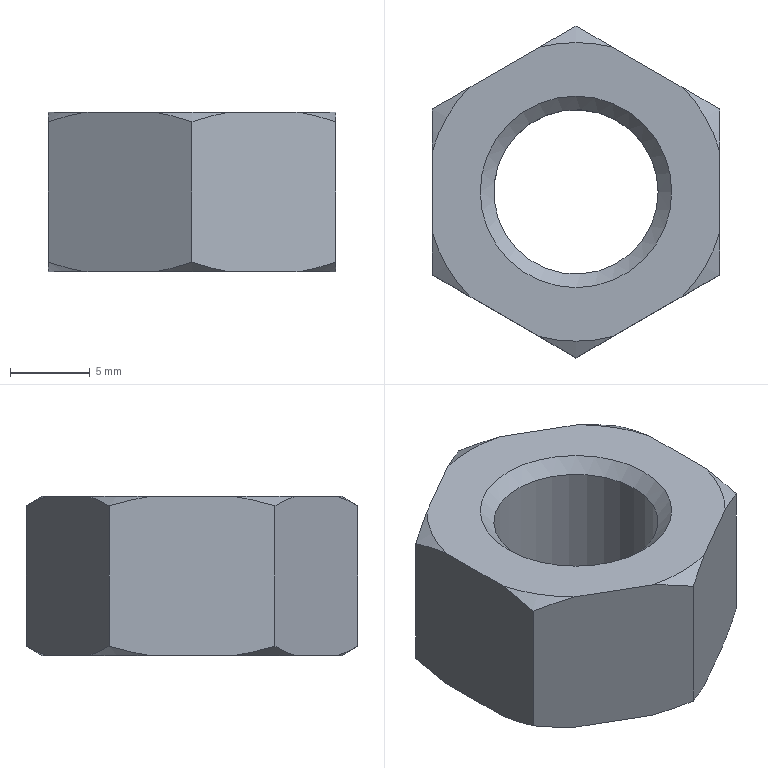Part | NX | features DATUM_CSYS 3, EXTRACT_FACE 2, EXTRACT_STRING 2, SKETCH 2, SWP104 2, EXTRUDE 1, HOLE PACKAGE 1, Instance Feature 1, Mirror Feature 1, SIMPLE HOLE 1, SYMBOLIC_THREAD 1 | 1 solid | 23 faces | box 18 x 20.785 x 10 mm | volume 1943 mm3 | cone 14 | plane 8 | cylinder 1 | commonest cylinder face diameters 10.3 x1
STEP:
#1=CARTESIAN_POINT('',(6.,0.,-10.));
#2=VERTEX_POINT('',#1);
#3=CARTESIAN_POINT('',(0.,0.,-10.));
#4=DIRECTION('',(0.,0.,1.));
#5=DIRECTION('',(1.,0.,0.));
#6=AXIS2_PLACEMENT_3D('',#3,#4,#5);
#7=CIRCLE('',#6,6.);
#8=EDGE_CURVE('',#2,#2,#7,.T.);
#9=ORIENTED_EDGE('',*,*,#8,.T.);
#10=EDGE_LOOP('',(#9));
#11=FACE_BOUND('',#10,.T.);
#12=CARTESIAN_POINT('',(9.,2.546,-10.));
#13=VERTEX_POINT('',#12);
#14=CARTESIAN_POINT('',(6.705,6.521,-10.));
#15=VERTEX_POINT('',#14);
#16=CARTESIAN_POINT('',(0.,0.,-10.));
#17=DIRECTION('',(0.,0.,1.));
#18=DIRECTION('',(1.,0.,0.));
#19=AXIS2_PLACEMENT_3D('',#16,#17,#18);
#20=CIRCLE('',#19,9.353);
#21=EDGE_CURVE('',#13,#15,#20,.T.);
#22=ORIENTED_EDGE('',*,*,#21,.F.);
#23=CARTESIAN_POINT('',(9.,-2.546,-10.));
#24=VERTEX_POINT('',#23);
#25=CARTESIAN_POINT('',(9.,-5.196,-10.));
#26=DIRECTION('',(0.,1.,0.));
#27=VECTOR('',#26,1000.);
#28=LINE('',#25,#27);
#29=EDGE_CURVE('',#24,#13,#28,.T.);
#30=ORIENTED_EDGE('',*,*,#29,.F.);
#31=CARTESIAN_POINT('',(6.705,-6.521,-10.));
#32=VERTEX_POINT('',#31);
#33=CARTESIAN_POINT('',(0.,0.,-10.));
#34=DIRECTION('',(0.,0.,1.));
#35=DIRECTION('',(1.,0.,0.));
#36=AXIS2_PLACEMENT_3D('',#33,#34,#35);
#37=CIRCLE('',#36,9.353);
#38=EDGE_CURVE('',#32,#24,#37,.T.);
#39=ORIENTED_EDGE('',*,*,#38,.F.);
#40=CARTESIAN_POINT('',(2.295,-9.067,-10.));
#41=VERTEX_POINT('',#40);
#42=CARTESIAN_POINT('',(0.,-10.392,-10.));
#43=DIRECTION('',(0.866,0.5,0.));
#44=VECTOR('',#43,1000.);
#45=LINE('',#42,#44);
#46=EDGE_CURVE('',#41,#32,#45,.T.);
#47=ORIENTED_EDGE('',*,*,#46,.F.);
#48=CARTESIAN_POINT('',(-2.295,-9.067,-10.));
#49=VERTEX_POINT('',#48);
#50=CARTESIAN_POINT('',(0.,0.,-10.));
#51=DIRECTION('',(0.,0.,1.));
#52=DIRECTION('',(1.,0.,0.));
#53=AXIS2_PLACEMENT_3D('',#50,#51,#52);
#54=CIRCLE('',#53,9.353);
#55=EDGE_CURVE('',#49,#41,#54,.T.);
#56=ORIENTED_EDGE('',*,*,#55,.F.);
#57=CARTESIAN_POINT('',(-6.705,-6.521,-10.));
#58=VERTEX_POINT('',#57);
#59=CARTESIAN_POINT('',(-9.,-5.196,-10.));
#60=DIRECTION('',(0.866,-0.5,0.));
#61=VECTOR('',#60,1000.);
#62=LINE('',#59,#61);
#63=EDGE_CURVE('',#58,#49,#62,.T.);
#64=ORIENTED_EDGE('',*,*,#63,.F.);
#65=CARTESIAN_POINT('',(-9.,-2.546,-10.));
#66=VERTEX_POINT('',#65);
#67=CARTESIAN_POINT('',(0.,0.,-10.));
#68=DIRECTION('',(0.,0.,1.));
#69=DIRECTION('',(1.,0.,0.));
#70=AXIS2_PLACEMENT_3D('',#67,#68,#69);
#71=CIRCLE('',#70,9.353);
#72=EDGE_CURVE('',#66,#58,#71,.T.);
#73=ORIENTED_EDGE('',*,*,#72,.F.);
#74=CARTESIAN_POINT('',(-9.,2.546,-10.));
#75=VERTEX_POINT('',#74);
#76=CARTESIAN_POINT('',(-9.,5.196,-10.));
#77=DIRECTION('',(0.,-1.,0.));
#78=VECTOR('',#77,1000.);
#79=LINE('',#76,#78);
#80=EDGE_CURVE('',#75,#66,#79,.T.);
#81=ORIENTED_EDGE('',*,*,#80,.F.);
#82=CARTESIAN_POINT('',(-6.705,6.521,-10.));
#83=VERTEX_POINT('',#82);
#84=CARTESIAN_POINT('',(0.,0.,-10.));
#85=DIRECTION('',(0.,0.,1.));
#86=DIRECTION('',(1.,0.,0.));
#87=AXIS2_PLACEMENT_3D('',#84,#85,#86);
#88=CIRCLE('',#87,9.353);
#89=EDGE_CURVE('',#83,#75,#88,.T.);
#90=ORIENTED_EDGE('',*,*,#89,.F.);
#91=CARTESIAN_POINT('',(-2.295,9.067,-10.));
#92=VERTEX_POINT('',#91);
#93=CARTESIAN_POINT('',(0.,10.392,-10.));
#94=DIRECTION('',(-0.866,-0.5,0.));
#95=VECTOR('',#94,1000.);
#96=LINE('',#93,#95);
#97=EDGE_CURVE('',#92,#83,#96,.T.);
#98=ORIENTED_EDGE('',*,*,#97,.F.);
#99=CARTESIAN_POINT('',(2.295,9.067,-10.));
#100=VERTEX_POINT('',#99);
#101=CARTESIAN_POINT('',(0.,0.,-10.));
#102=DIRECTION('',(0.,0.,1.));
#103=DIRECTION('',(1.,0.,0.));
#104=AXIS2_PLACEMENT_3D('',#101,#102,#103);
#105=CIRCLE('',#104,9.353);
#106=EDGE_CURVE('',#100,#92,#105,.T.);
#107=ORIENTED_EDGE('',*,*,#106,.F.);
#108=CARTESIAN_POINT('',(9.,5.196,-10.));
#109=DIRECTION('',(-0.866,0.5,0.));
#110=VECTOR('',#109,1000.);
#111=LINE('',#108,#110);
#112=EDGE_CURVE('',#15,#100,#111,.T.);
#113=ORIENTED_EDGE('',*,*,#112,.F.);
#114=EDGE_LOOP('',(#22,#30,#39,#47,#56,#64,#73,#81,#90,#98,#107,#113));
#115=FACE_BOUND('',#114,.T.);
#116=CARTESIAN_POINT('',(0.,0.,-10.));
#117=DIRECTION('',(0.,0.,1.));
#118=DIRECTION('',(1.,0.,0.));
#119=AXIS2_PLACEMENT_3D('',#116,#117,#118);
#120=PLANE('',#119);
#121=ADVANCED_FACE('',(#11,#115),#120,.F.);
#122=CARTESIAN_POINT('',(-9.,-5.196,-9.4));
#123=VERTEX_POINT('',#122);
#124=CARTESIAN_POINT('',(-9.,-5.196,-9.4));
#125=CARTESIAN_POINT('',(-9.,-4.328,-9.65));
#126=CARTESIAN_POINT('',(-9.,-3.439,-9.86));
#127=CARTESIAN_POINT('',(-9.,-2.546,-10.));
#128=B_SPLINE_CURVE_WITH_KNOTS('',3,(#124,#125,#126,#127),.UNSPECIFIED.,.F.,.F.,(4,4),(0.00669,0.009395),.UNSPECIFIED.);
#129=EDGE_CURVE('',#123,#66,#128,.T.);
#130=ORIENTED_EDGE('',*,*,#129,.F.);
#131=CARTESIAN_POINT('',(-9.,-5.196,-0.6));
#132=VERTEX_POINT('',#131);
#133=CARTESIAN_POINT('',(-9.,-5.196,-10.));
#134=DIRECTION('',(0.,0.,1.));
#135=VECTOR('',#134,1000.);
#136=LINE('',#133,#135);
#137=EDGE_CURVE('',#123,#132,#136,.T.);
#138=ORIENTED_EDGE('',*,*,#137,.T.);
#139=CARTESIAN_POINT('',(-9.,-2.546,0.));
#140=VERTEX_POINT('',#139);
#141=CARTESIAN_POINT('',(-9.,-2.546,0.));
#142=CARTESIAN_POINT('',(-9.,-3.446,-0.1415));
#143=CARTESIAN_POINT('',(-9.,-4.33,-0.3499));
#144=CARTESIAN_POINT('',(-9.,-5.196,-0.6));
#145=B_SPLINE_CURVE_WITH_KNOTS('',3,(#141,#142,#143,#144),.UNSPECIFIED.,.F.,.F.,(4,4),(0.01452,0.01723),.UNSPECIFIED.);
#146=EDGE_CURVE('',#140,#132,#145,.T.);
#147=ORIENTED_EDGE('',*,*,#146,.F.);
#148=CARTESIAN_POINT('',(-9.,2.546,0.));
#149=VERTEX_POINT('',#148);
#150=CARTESIAN_POINT('',(-9.,5.196,0.));
#151=DIRECTION('',(0.,-1.,0.));
#152=VECTOR('',#151,1000.);
#153=LINE('',#150,#152);
#154=EDGE_CURVE('',#149,#140,#153,.T.);
#155=ORIENTED_EDGE('',*,*,#154,.F.);
#156=CARTESIAN_POINT('',(-9.,5.196,-0.6));
#157=VERTEX_POINT('',#156);
#158=CARTESIAN_POINT('',(-9.,5.196,-0.6));
#159=CARTESIAN_POINT('',(-9.,4.328,-0.3495));
#160=CARTESIAN_POINT('',(-9.,3.439,-0.1403));
#161=CARTESIAN_POINT('',(-9.,2.546,0.));
#162=B_SPLINE_CURVE_WITH_KNOTS('',3,(#158,#159,#160,#161),.UNSPECIFIED.,.F.,.F.,(4,4),(0.00669,0.009395),.UNSPECIFIED.);
#163=EDGE_CURVE('',#157,#149,#162,.T.);
#164=ORIENTED_EDGE('',*,*,#163,.F.);
#165=CARTESIAN_POINT('',(-9.,5.196,-9.4));
#166=VERTEX_POINT('',#165);
#167=CARTESIAN_POINT('',(-9.,5.196,-10.));
#168=DIRECTION('',(0.,0.,1.));
#169=VECTOR('',#168,1000.);
#170=LINE('',#167,#169);
#171=EDGE_CURVE('',#166,#157,#170,.T.);
#172=ORIENTED_EDGE('',*,*,#171,.F.);
#173=CARTESIAN_POINT('',(-9.,2.546,-10.));
#174=CARTESIAN_POINT('',(-9.,3.446,-9.859));
#175=CARTESIAN_POINT('',(-9.,4.33,-9.65));
#176=CARTESIAN_POINT('',(-9.,5.196,-9.4));
#177=B_SPLINE_CURVE_WITH_KNOTS('',3,(#173,#174,#175,#176),.UNSPECIFIED.,.F.,.F.,(4,4),(0.01452,0.01723),.UNSPECIFIED.);
#178=EDGE_CURVE('',#75,#166,#177,.T.);
#179=ORIENTED_EDGE('',*,*,#178,.F.);
#180=ORIENTED_EDGE('',*,*,#80,.T.);
#181=EDGE_LOOP('',(#130,#138,#147,#155,#164,#172,#179,#180));
#182=FACE_BOUND('',#181,.T.);
#183=CARTESIAN_POINT('',(-9.,5.196,-10.));
#184=DIRECTION('',(-1.,0.,0.));
#185=DIRECTION('',(0.,-1.,0.));
#186=AXIS2_PLACEMENT_3D('',#183,#184,#185);
#187=PLANE('',#186);
#188=ADVANCED_FACE('',(#182),#187,.T.);
#189=CARTESIAN_POINT('',(0.,-10.392,-9.4));
#190=VERTEX_POINT('',#189);
#191=CARTESIAN_POINT('',(0.,-10.392,-9.4));
#192=CARTESIAN_POINT('',(-0.7544,-9.957,-9.651));
#193=CARTESIAN_POINT('',(-1.525,-9.512,-9.86));
#194=CARTESIAN_POINT('',(-2.295,-9.067,-10.));
#195=B_SPLINE_CURVE_WITH_KNOTS('',3,(#191,#192,#193,#194),.UNSPECIFIED.,.F.,.F.,(4,4),(0.007754,0.01047),.UNSPECIFIED.);
#196=EDGE_CURVE('',#190,#49,#195,.T.);
#197=ORIENTED_EDGE('',*,*,#196,.F.);
#198=CARTESIAN_POINT('',(0.,-10.392,-0.6));
#199=VERTEX_POINT('',#198);
#200=CARTESIAN_POINT('',(0.,-10.392,-10.));
#201=DIRECTION('',(0.,0.,1.));
#202=VECTOR('',#201,1000.);
#203=LINE('',#200,#202);
#204=EDGE_CURVE('',#190,#199,#203,.T.);
#205=ORIENTED_EDGE('',*,*,#204,.T.);
#206=CARTESIAN_POINT('',(-2.295,-9.067,0.));
#207=VERTEX_POINT('',#206);
#208=CARTESIAN_POINT('',(-2.295,-9.067,0.));
#209=CARTESIAN_POINT('',(-1.515,-9.517,-0.1416));
#210=CARTESIAN_POINT('',(-0.7521,-9.958,-0.3493));
#211=CARTESIAN_POINT('',(0.,-10.392,-0.6));
#212=B_SPLINE_CURVE_WITH_KNOTS('',3,(#208,#209,#210,#211),.UNSPECIFIED.,.F.,.F.,(4,4),(0.01558,0.01831),.UNSPECIFIED.);
#213=EDGE_CURVE('',#207,#199,#212,.T.);
#214=ORIENTED_EDGE('',*,*,#213,.F.);
#215=CARTESIAN_POINT('',(-6.705,-6.521,0.));
#216=VERTEX_POINT('',#215);
#217=CARTESIAN_POINT('',(-9.,-5.196,0.));
#218=DIRECTION('',(0.866,-0.5,0.));
#219=VECTOR('',#218,1000.);
#220=LINE('',#217,#219);
#221=EDGE_CURVE('',#216,#207,#220,.T.);
#222=ORIENTED_EDGE('',*,*,#221,.F.);
#223=CARTESIAN_POINT('',(-9.,-5.196,-0.6));
#224=CARTESIAN_POINT('',(-8.246,-5.632,-0.3485));
#225=CARTESIAN_POINT('',(-7.475,-6.076,-0.1398));
#226=CARTESIAN_POINT('',(-6.705,-6.521,0.));
#227=B_SPLINE_CURVE_WITH_KNOTS('',3,(#223,#224,#225,#226),.UNSPECIFIED.,.F.,.F.,(4,4),(0.007754,0.01047),.UNSPECIFIED.);
#228=EDGE_CURVE('',#132,#216,#227,.T.);
#229=ORIENTED_EDGE('',*,*,#228,.F.);
#230=ORIENTED_EDGE('',*,*,#137,.F.);
#231=CARTESIAN_POINT('',(-6.705,-6.521,-10.));
#232=CARTESIAN_POINT('',(-7.485,-6.071,-9.858));
#233=CARTESIAN_POINT('',(-8.248,-5.63,-9.651));
#234=CARTESIAN_POINT('',(-9.,-5.196,-9.4));
#235=B_SPLINE_CURVE_WITH_KNOTS('',3,(#231,#232,#233,#234),.UNSPECIFIED.,.F.,.F.,(4,4),(0.01558,0.01831),.UNSPECIFIED.);
#236=EDGE_CURVE('',#58,#123,#235,.T.);
#237=ORIENTED_EDGE('',*,*,#236,.F.);
#238=ORIENTED_EDGE('',*,*,#63,.T.);
#239=EDGE_LOOP('',(#197,#205,#214,#222,#229,#230,#237,#238));
#240=FACE_BOUND('',#239,.T.);
#241=CARTESIAN_POINT('',(-9.,-5.196,-10.));
#242=DIRECTION('',(-0.5,-0.866,0.));
#243=DIRECTION('',(0.866,-0.5,0.));
#244=AXIS2_PLACEMENT_3D('',#241,#242,#243);
#245=PLANE('',#244);
#246=ADVANCED_FACE('',(#240),#245,.T.);
#247=CARTESIAN_POINT('',(9.,-5.196,-9.4));
#248=VERTEX_POINT('',#247);
#249=CARTESIAN_POINT('',(9.,-5.196,-9.4));
#250=CARTESIAN_POINT('',(8.246,-5.632,-9.651));
#251=CARTESIAN_POINT('',(7.475,-6.076,-9.86));
#252=CARTESIAN_POINT('',(6.705,-6.521,-10.));
#253=B_SPLINE_CURVE_WITH_KNOTS('',3,(#249,#250,#251,#252),.UNSPECIFIED.,.F.,.F.,(4,4),(0.007754,0.01047),.UNSPECIFIED.);
#254=EDGE_CURVE('',#248,#32,#253,.T.);
#255=ORIENTED_EDGE('',*,*,#254,.F.);
#256=CARTESIAN_POINT('',(9.,-5.196,-0.6));
#257=VERTEX_POINT('',#256);
#258=CARTESIAN_POINT('',(9.,-5.196,-10.));
#259=DIRECTION('',(0.,0.,1.));
#260=VECTOR('',#259,1000.);
#261=LINE('',#258,#260);
#262=EDGE_CURVE('',#248,#257,#261,.T.);
#263=ORIENTED_EDGE('',*,*,#262,.T.);
#264=CARTESIAN_POINT('',(6.705,-6.521,0.));
#265=VERTEX_POINT('',#264);
#266=CARTESIAN_POINT('',(6.705,-6.521,0.));
#267=CARTESIAN_POINT('',(7.485,-6.071,-0.1416));
#268=CARTESIAN_POINT('',(8.248,-5.63,-0.3493));
#269=CARTESIAN_POINT('',(9.,-5.196,-0.6));
#270=B_SPLINE_CURVE_WITH_KNOTS('',3,(#266,#267,#268,#269),.UNSPECIFIED.,.F.,.F.,(4,4),(0.01558,0.01831),.UNSPECIFIED.);
#271=EDGE_CURVE('',#265,#257,#270,.T.);
#272=ORIENTED_EDGE('',*,*,#271,.F.);
#273=CARTESIAN_POINT('',(2.295,-9.067,0.));
#274=VERTEX_POINT('',#273);
#275=CARTESIAN_POINT('',(0.,-10.392,0.));
#276=DIRECTION('',(0.866,0.5,0.));
#277=VECTOR('',#276,1000.);
#278=LINE('',#275,#277);
#279=EDGE_CURVE('',#274,#265,#278,.T.);
#280=ORIENTED_EDGE('',*,*,#279,.F.);
#281=CARTESIAN_POINT('',(0.,-10.392,-0.6));
#282=CARTESIAN_POINT('',(0.7544,-9.957,-0.3485));
#283=CARTESIAN_POINT('',(1.525,-9.512,-0.1398));
#284=CARTESIAN_POINT('',(2.295,-9.067,0.));
#285=B_SPLINE_CURVE_WITH_KNOTS('',3,(#281,#282,#283,#284),.UNSPECIFIED.,.F.,.F.,(4,4),(0.007754,0.01047),.UNSPECIFIED.);
#286=EDGE_CURVE('',#199,#274,#285,.T.);
#287=ORIENTED_EDGE('',*,*,#286,.F.);
#288=ORIENTED_EDGE('',*,*,#204,.F.);
#289=CARTESIAN_POINT('',(2.295,-9.067,-10.));
#290=CARTESIAN_POINT('',(1.515,-9.517,-9.858));
#291=CARTESIAN_POINT('',(0.7521,-9.958,-9.651));
#292=CARTESIAN_POINT('',(0.,-10.392,-9.4));
#293=B_SPLINE_CURVE_WITH_KNOTS('',3,(#289,#290,#291,#292),.UNSPECIFIED.,.F.,.F.,(4,4),(0.01558,0.01831),.UNSPECIFIED.);
#294=EDGE_CURVE('',#41,#190,#293,.T.);
#295=ORIENTED_EDGE('',*,*,#294,.F.);
#296=ORIENTED_EDGE('',*,*,#46,.T.);
#297=EDGE_LOOP('',(#255,#263,#272,#280,#287,#288,#295,#296));
#298=FACE_BOUND('',#297,.T.);
#299=CARTESIAN_POINT('',(0.,-10.392,-10.));
#300=DIRECTION('',(0.5,-0.866,0.));
#301=DIRECTION('',(0.866,0.5,0.));
#302=AXIS2_PLACEMENT_3D('',#299,#300,#301);
#303=PLANE('',#302);
#304=ADVANCED_FACE('',(#298),#303,.T.);
#305=CARTESIAN_POINT('',(9.,5.196,-9.4));
#306=VERTEX_POINT('',#305);
#307=CARTESIAN_POINT('',(9.,5.196,-9.4));
#308=CARTESIAN_POINT('',(9.,4.328,-9.65));
#309=CARTESIAN_POINT('',(9.,3.439,-9.86));
#310=CARTESIAN_POINT('',(9.,2.546,-10.));
#311=B_SPLINE_CURVE_WITH_KNOTS('',3,(#307,#308,#309,#310),.UNSPECIFIED.,.F.,.F.,(4,4),(0.00669,0.009395),.UNSPECIFIED.);
#312=EDGE_CURVE('',#306,#13,#311,.T.);
#313=ORIENTED_EDGE('',*,*,#312,.F.);
#314=CARTESIAN_POINT('',(9.,5.196,-0.6));
#315=VERTEX_POINT('',#314);
#316=CARTESIAN_POINT('',(9.,5.196,-10.));
#317=DIRECTION('',(0.,0.,1.));
#318=VECTOR('',#317,1000.);
#319=LINE('',#316,#318);
#320=EDGE_CURVE('',#306,#315,#319,.T.);
#321=ORIENTED_EDGE('',*,*,#320,.T.);
#322=CARTESIAN_POINT('',(9.,2.546,0.));
#323=VERTEX_POINT('',#322);
#324=CARTESIAN_POINT('',(9.,2.546,0.));
#325=CARTESIAN_POINT('',(9.,3.446,-0.1415));
#326=CARTESIAN_POINT('',(9.,4.33,-0.3499));
#327=CARTESIAN_POINT('',(9.,5.196,-0.6));
#328=B_SPLINE_CURVE_WITH_KNOTS('',3,(#324,#325,#326,#327),.UNSPECIFIED.,.F.,.F.,(4,4),(0.01452,0.01723),.UNSPECIFIED.);
#329=EDGE_CURVE('',#323,#315,#328,.T.);
#330=ORIENTED_EDGE('',*,*,#329,.F.);
#331=CARTESIAN_POINT('',(9.,-2.546,0.));
#332=VERTEX_POINT('',#331);
#333=CARTESIAN_POINT('',(9.,-5.196,0.));
#334=DIRECTION('',(0.,1.,0.));
#335=VECTOR('',#334,1000.);
#336=LINE('',#333,#335);
#337=EDGE_CURVE('',#332,#323,#336,.T.);
#338=ORIENTED_EDGE('',*,*,#337,.F.);
#339=CARTESIAN_POINT('',(9.,-5.196,-0.6));
#340=CARTESIAN_POINT('',(9.,-4.328,-0.3495));
#341=CARTESIAN_POINT('',(9.,-3.439,-0.1403));
#342=CARTESIAN_POINT('',(9.,-2.546,0.));
#343=B_SPLINE_CURVE_WITH_KNOTS('',3,(#339,#340,#341,#342),.UNSPECIFIED.,.F.,.F.,(4,4),(0.00669,0.009395),.UNSPECIFIED.);
#344=EDGE_CURVE('',#257,#332,#343,.T.);
#345=ORIENTED_EDGE('',*,*,#344,.F.);
#346=ORIENTED_EDGE('',*,*,#262,.F.);
#347=CARTESIAN_POINT('',(9.,-2.546,-10.));
#348=CARTESIAN_POINT('',(9.,-3.446,-9.859));
#349=CARTESIAN_POINT('',(9.,-4.33,-9.65));
#350=CARTESIAN_POINT('',(9.,-5.196,-9.4));
#351=B_SPLINE_CURVE_WITH_KNOTS('',3,(#347,#348,#349,#350),.UNSPECIFIED.,.F.,.F.,(4,4),(0.01452,0.01723),.UNSPECIFIED.);
#352=EDGE_CURVE('',#24,#248,#351,.T.);
#353=ORIENTED_EDGE('',*,*,#352,.F.);
#354=ORIENTED_EDGE('',*,*,#29,.T.);
#355=EDGE_LOOP('',(#313,#321,#330,#338,#345,#346,#353,#354));
#356=FACE_BOUND('',#355,.T.);
#357=CARTESIAN_POINT('',(9.,-5.196,-10.));
#358=DIRECTION('',(1.,0.,0.));
#359=DIRECTION('',(0.,1.,0.));
#360=AXIS2_PLACEMENT_3D('',#357,#358,#359);
#361=PLANE('',#360);
#362=ADVANCED_FACE('',(#356),#361,.T.);
#363=CARTESIAN_POINT('',(0.,10.392,-9.4));
#364=VERTEX_POINT('',#363);
#365=CARTESIAN_POINT('',(0.,10.392,-9.4));
#366=CARTESIAN_POINT('',(0.7544,9.957,-9.651));
#367=CARTESIAN_POINT('',(1.525,9.512,-9.86));
#368=CARTESIAN_POINT('',(2.295,9.067,-10.));
#369=B_SPLINE_CURVE_WITH_KNOTS('',3,(#365,#366,#367,#368),.UNSPECIFIED.,.F.,.F.,(4,4),(0.007754,0.01047),.UNSPECIFIED.);
#370=EDGE_CURVE('',#364,#100,#369,.T.);
#371=ORIENTED_EDGE('',*,*,#370,.F.);
#372=CARTESIAN_POINT('',(0.,10.392,-0.6));
#373=VERTEX_POINT('',#372);
#374=CARTESIAN_POINT('',(0.,10.392,-10.));
#375=DIRECTION('',(0.,0.,1.));
#376=VECTOR('',#375,1000.);
#377=LINE('',#374,#376);
#378=EDGE_CURVE('',#364,#373,#377,.T.);
#379=ORIENTED_EDGE('',*,*,#378,.T.);
#380=CARTESIAN_POINT('',(2.295,9.067,0.));
#381=VERTEX_POINT('',#380);
#382=CARTESIAN_POINT('',(2.295,9.067,0.));
#383=CARTESIAN_POINT('',(1.515,9.517,-0.1416));
#384=CARTESIAN_POINT('',(0.7521,9.958,-0.3493));
#385=CARTESIAN_POINT('',(0.,10.392,-0.6));
#386=B_SPLINE_CURVE_WITH_KNOTS('',3,(#382,#383,#384,#385),.UNSPECIFIED.,.F.,.F.,(4,4),(0.01558,0.01831),.UNSPECIFIED.);
#387=EDGE_CURVE('',#381,#373,#386,.T.);
#388=ORIENTED_EDGE('',*,*,#387,.F.);
#389=CARTESIAN_POINT('',(6.705,6.521,0.));
#390=VERTEX_POINT('',#389);
#391=CARTESIAN_POINT('',(9.,5.196,0.));
#392=DIRECTION('',(-0.866,0.5,0.));
#393=VECTOR('',#392,1000.);
#394=LINE('',#391,#393);
#395=EDGE_CURVE('',#390,#381,#394,.T.);
#396=ORIENTED_EDGE('',*,*,#395,.F.);
#397=CARTESIAN_POINT('',(9.,5.196,-0.6));
#398=CARTESIAN_POINT('',(8.246,5.632,-0.3485));
#399=CARTESIAN_POINT('',(7.475,6.076,-0.1398));
#400=CARTESIAN_POINT('',(6.705,6.521,0.));
#401=B_SPLINE_CURVE_WITH_KNOTS('',3,(#397,#398,#399,#400),.UNSPECIFIED.,.F.,.F.,(4,4),(0.007754,0.01047),.UNSPECIFIED.);
#402=EDGE_CURVE('',#315,#390,#401,.T.);
#403=ORIENTED_EDGE('',*,*,#402,.F.);
#404=ORIENTED_EDGE('',*,*,#320,.F.);
#405=CARTESIAN_POINT('',(6.705,6.521,-10.));
#406=CARTESIAN_POINT('',(7.485,6.071,-9.858));
#407=CARTESIAN_POINT('',(8.248,5.63,-9.651));
#408=CARTESIAN_POINT('',(9.,5.196,-9.4));
#409=B_SPLINE_CURVE_WITH_KNOTS('',3,(#405,#406,#407,#408),.UNSPECIFIED.,.F.,.F.,(4,4),(0.01558,0.01831),.UNSPECIFIED.);
#410=EDGE_CURVE('',#15,#306,#409,.T.);
#411=ORIENTED_EDGE('',*,*,#410,.F.);
#412=ORIENTED_EDGE('',*,*,#112,.T.);
#413=EDGE_LOOP('',(#371,#379,#388,#396,#403,#404,#411,#412));
#414=FACE_BOUND('',#413,.T.);
#415=CARTESIAN_POINT('',(9.,5.196,-10.));
#416=DIRECTION('',(0.5,0.866,0.));
#417=DIRECTION('',(-0.866,0.5,0.));
#418=AXIS2_PLACEMENT_3D('',#415,#416,#417);
#419=PLANE('',#418);
#420=ADVANCED_FACE('',(#414),#419,.T.);
#421=CARTESIAN_POINT('',(-9.,5.196,-9.4));
#422=CARTESIAN_POINT('',(-8.246,5.632,-9.651));
#423=CARTESIAN_POINT('',(-7.475,6.076,-9.86));
#424=CARTESIAN_POINT('',(-6.705,6.521,-10.));
#425=B_SPLINE_CURVE_WITH_KNOTS('',3,(#421,#422,#423,#424),.UNSPECIFIED.,.F.,.F.,(4,4),(0.007754,0.01047),.UNSPECIFIED.);
#426=EDGE_CURVE('',#166,#83,#425,.T.);
#427=ORIENTED_EDGE('',*,*,#426,.F.);
#428=ORIENTED_EDGE('',*,*,#171,.T.);
#429=CARTESIAN_POINT('',(-6.705,6.521,0.));
#430=VERTEX_POINT('',#429);
#431=CARTESIAN_POINT('',(-6.705,6.521,0.));
#432=CARTESIAN_POINT('',(-7.485,6.071,-0.1416));
#433=CARTESIAN_POINT('',(-8.248,5.63,-0.3493));
#434=CARTESIAN_POINT('',(-9.,5.196,-0.6));
#435=B_SPLINE_CURVE_WITH_KNOTS('',3,(#431,#432,#433,#434),.UNSPECIFIED.,.F.,.F.,(4,4),(0.01558,0.01831),.UNSPECIFIED.);
#436=EDGE_CURVE('',#430,#157,#435,.T.);
#437=ORIENTED_EDGE('',*,*,#436,.F.);
#438=CARTESIAN_POINT('',(-2.295,9.067,0.));
#439=VERTEX_POINT('',#438);
#440=CARTESIAN_POINT('',(0.,10.392,0.));
#441=DIRECTION('',(-0.866,-0.5,0.));
#442=VECTOR('',#441,1000.);
#443=LINE('',#440,#442);
#444=EDGE_CURVE('',#439,#430,#443,.T.);
#445=ORIENTED_EDGE('',*,*,#444,.F.);
#446=CARTESIAN_POINT('',(0.,10.392,-0.6));
#447=CARTESIAN_POINT('',(-0.7544,9.957,-0.3485));
#448=CARTESIAN_POINT('',(-1.525,9.512,-0.1398));
#449=CARTESIAN_POINT('',(-2.295,9.067,0.));
#450=B_SPLINE_CURVE_WITH_KNOTS('',3,(#446,#447,#448,#449),.UNSPECIFIED.,.F.,.F.,(4,4),(0.007754,0.01047),.UNSPECIFIED.);
#451=EDGE_CURVE('',#373,#439,#450,.T.);
#452=ORIENTED_EDGE('',*,*,#451,.F.);
#453=ORIENTED_EDGE('',*,*,#378,.F.);
#454=CARTESIAN_POINT('',(-2.295,9.067,-10.));
#455=CARTESIAN_POINT('',(-1.515,9.517,-9.858));
#456=CARTESIAN_POINT('',(-0.7521,9.958,-9.651));
#457=CARTESIAN_POINT('',(0.,10.392,-9.4));
#458=B_SPLINE_CURVE_WITH_KNOTS('',3,(#454,#455,#456,#457),.UNSPECIFIED.,.F.,.F.,(4,4),(0.01558,0.01831),.UNSPECIFIED.);
#459=EDGE_CURVE('',#92,#364,#458,.T.);
#460=ORIENTED_EDGE('',*,*,#459,.F.);
#461=ORIENTED_EDGE('',*,*,#97,.T.);
#462=EDGE_LOOP('',(#427,#428,#437,#445,#452,#453,#460,#461));
#463=FACE_BOUND('',#462,.T.);
#464=CARTESIAN_POINT('',(0.,10.392,-10.));
#465=DIRECTION('',(-0.5,0.866,0.));
#466=DIRECTION('',(-0.866,-0.5,0.));
#467=AXIS2_PLACEMENT_3D('',#464,#465,#466);
#468=PLANE('',#467);
#469=ADVANCED_FACE('',(#463),#468,.T.);
#470=CARTESIAN_POINT('',(6.,0.,0.));
#471=VERTEX_POINT('',#470);
#472=CARTESIAN_POINT('',(0.,0.,0.));
#473=DIRECTION('',(0.,0.,1.));
#474=DIRECTION('',(1.,0.,0.));
#475=AXIS2_PLACEMENT_3D('',#472,#473,#474);
#476=CIRCLE('',#475,6.);
#477=EDGE_CURVE('',#471,#471,#476,.F.);
#478=ORIENTED_EDGE('',*,*,#477,.T.);
#479=EDGE_LOOP('',(#478));
#480=FACE_BOUND('',#479,.T.);
#481=CARTESIAN_POINT('',(0.,0.,0.));
#482=DIRECTION('',(0.,0.,-1.));
#483=DIRECTION('',(-1.,0.,0.));
#484=AXIS2_PLACEMENT_3D('',#481,#482,#483);
#485=CIRCLE('',#484,9.353);
#486=EDGE_CURVE('',#149,#430,#485,.T.);
#487=ORIENTED_EDGE('',*,*,#486,.F.);
#488=ORIENTED_EDGE('',*,*,#154,.T.);
#489=CARTESIAN_POINT('',(0.,0.,0.));
#490=DIRECTION('',(0.,0.,-1.));
#491=DIRECTION('',(-1.,0.,0.));
#492=AXIS2_PLACEMENT_3D('',#489,#490,#491);
#493=CIRCLE('',#492,9.353);
#494=EDGE_CURVE('',#216,#140,#493,.T.);
#495=ORIENTED_EDGE('',*,*,#494,.F.);
#496=ORIENTED_EDGE('',*,*,#221,.T.);
#497=CARTESIAN_POINT('',(0.,0.,0.));
#498=DIRECTION('',(0.,0.,-1.));
#499=DIRECTION('',(-1.,0.,0.));
#500=AXIS2_PLACEMENT_3D('',#497,#498,#499);
#501=CIRCLE('',#500,9.353);
#502=EDGE_CURVE('',#274,#207,#501,.T.);
#503=ORIENTED_EDGE('',*,*,#502,.F.);
#504=ORIENTED_EDGE('',*,*,#279,.T.);
#505=CARTESIAN_POINT('',(0.,0.,0.));
#506=DIRECTION('',(0.,0.,-1.));
#507=DIRECTION('',(-1.,0.,0.));
#508=AXIS2_PLACEMENT_3D('',#505,#506,#507);
#509=CIRCLE('',#508,9.353);
#510=EDGE_CURVE('',#332,#265,#509,.T.);
#511=ORIENTED_EDGE('',*,*,#510,.F.);
#512=ORIENTED_EDGE('',*,*,#337,.T.);
#513=CARTESIAN_POINT('',(0.,0.,0.));
#514=DIRECTION('',(0.,0.,-1.));
#515=DIRECTION('',(-1.,0.,0.));
#516=AXIS2_PLACEMENT_3D('',#513,#514,#515);
#517=CIRCLE('',#516,9.353);
#518=EDGE_CURVE('',#390,#323,#517,.T.);
#519=ORIENTED_EDGE('',*,*,#518,.F.);
#520=ORIENTED_EDGE('',*,*,#395,.T.);
#521=CARTESIAN_POINT('',(0.,0.,0.));
#522=DIRECTION('',(0.,0.,-1.));
#523=DIRECTION('',(-1.,0.,0.));
#524=AXIS2_PLACEMENT_3D('',#521,#522,#523);
#525=CIRCLE('',#524,9.353);
#526=EDGE_CURVE('',#439,#381,#525,.T.);
#527=ORIENTED_EDGE('',*,*,#526,.F.);
#528=ORIENTED_EDGE('',*,*,#444,.T.);
#529=EDGE_LOOP('',(#487,#488,#495,#496,#503,#504,#511,#512,#519,#520,#527,#528));
#530=FACE_BOUND('',#529,.T.);
#531=CARTESIAN_POINT('',(0.,0.,0.));
#532=DIRECTION('',(0.,0.,1.));
#533=DIRECTION('',(1.,0.,0.));
#534=AXIS2_PLACEMENT_3D('',#531,#532,#533);
#535=PLANE('',#534);
#536=ADVANCED_FACE('',(#480,#530),#535,.T.);
#537=ORIENTED_EDGE('',*,*,#163,.T.);
#538=ORIENTED_EDGE('',*,*,#486,.T.);
#539=ORIENTED_EDGE('',*,*,#436,.T.);
#540=EDGE_LOOP('',(#537,#538,#539));
#541=FACE_BOUND('',#540,.T.);
#542=CARTESIAN_POINT('',(0.,0.,0.));
#543=DIRECTION('',(0.,0.,-1.));
#544=DIRECTION('',(-1.,0.,0.));
#545=AXIS2_PLACEMENT_3D('',#542,#543,#544);
#546=CONICAL_SURFACE('',#545,9.353,1.047);
#547=ADVANCED_FACE('',(#541),#546,.T.);
#548=ORIENTED_EDGE('',*,*,#387,.T.);
#549=ORIENTED_EDGE('',*,*,#451,.T.);
#550=ORIENTED_EDGE('',*,*,#526,.T.);
#551=EDGE_LOOP('',(#548,#549,#550));
#552=FACE_BOUND('',#551,.T.);
#553=CARTESIAN_POINT('',(0.,0.,0.));
#554=DIRECTION('',(0.,0.,-1.));
#555=DIRECTION('',(-1.,0.,0.));
#556=AXIS2_PLACEMENT_3D('',#553,#554,#555);
#557=CONICAL_SURFACE('',#556,9.353,1.047);
#558=ADVANCED_FACE('',(#552),#557,.T.);
#559=ORIENTED_EDGE('',*,*,#329,.T.);
#560=ORIENTED_EDGE('',*,*,#402,.T.);
#561=ORIENTED_EDGE('',*,*,#518,.T.);
#562=EDGE_LOOP('',(#559,#560,#561));
#563=FACE_BOUND('',#562,.T.);
#564=CARTESIAN_POINT('',(0.,0.,0.));
#565=DIRECTION('',(0.,0.,-1.));
#566=DIRECTION('',(-1.,0.,0.));
#567=AXIS2_PLACEMENT_3D('',#564,#565,#566);
#568=CONICAL_SURFACE('',#567,9.353,1.047);
#569=ADVANCED_FACE('',(#563),#568,.T.);
#570=ORIENTED_EDGE('',*,*,#271,.T.);
#571=ORIENTED_EDGE('',*,*,#344,.T.);
#572=ORIENTED_EDGE('',*,*,#510,.T.);
#573=EDGE_LOOP('',(#570,#571,#572));
#574=FACE_BOUND('',#573,.T.);
#575=CARTESIAN_POINT('',(0.,0.,0.));
#576=DIRECTION('',(0.,0.,-1.));
#577=DIRECTION('',(-1.,0.,0.));
#578=AXIS2_PLACEMENT_3D('',#575,#576,#577);
#579=CONICAL_SURFACE('',#578,9.353,1.047);
#580=ADVANCED_FACE('',(#574),#579,.T.);
#581=ORIENTED_EDGE('',*,*,#213,.T.);
#582=ORIENTED_EDGE('',*,*,#286,.T.);
#583=ORIENTED_EDGE('',*,*,#502,.T.);
#584=EDGE_LOOP('',(#581,#582,#583));
#585=FACE_BOUND('',#584,.T.);
#586=CARTESIAN_POINT('',(0.,0.,0.));
#587=DIRECTION('',(0.,0.,-1.));
#588=DIRECTION('',(-1.,0.,0.));
#589=AXIS2_PLACEMENT_3D('',#586,#587,#588);
#590=CONICAL_SURFACE('',#589,9.353,1.047);
#591=ADVANCED_FACE('',(#585),#590,.T.);
#592=ORIENTED_EDGE('',*,*,#146,.T.);
#593=ORIENTED_EDGE('',*,*,#228,.T.);
#594=ORIENTED_EDGE('',*,*,#494,.T.);
#595=EDGE_LOOP('',(#592,#593,#594));
#596=FACE_BOUND('',#595,.T.);
#597=CARTESIAN_POINT('',(0.,0.,0.));
#598=DIRECTION('',(0.,0.,-1.));
#599=DIRECTION('',(-1.,0.,0.));
#600=AXIS2_PLACEMENT_3D('',#597,#598,#599);
#601=CONICAL_SURFACE('',#600,9.353,1.047);
#602=ADVANCED_FACE('',(#596),#601,.T.);
#603=ORIENTED_EDGE('',*,*,#370,.T.);
#604=ORIENTED_EDGE('',*,*,#106,.T.);
#605=ORIENTED_EDGE('',*,*,#459,.T.);
#606=EDGE_LOOP('',(#603,#604,#605));
#607=FACE_BOUND('',#606,.T.);
#608=CARTESIAN_POINT('',(0.,0.,-10.));
#609=DIRECTION('',(0.,0.,1.));
#610=DIRECTION('',(1.,0.,0.));
#611=AXIS2_PLACEMENT_3D('',#608,#609,#610);
#612=CONICAL_SURFACE('',#611,9.353,1.047);
#613=ADVANCED_FACE('',(#607),#612,.T.);
#614=ORIENTED_EDGE('',*,*,#178,.T.);
#615=ORIENTED_EDGE('',*,*,#426,.T.);
#616=ORIENTED_EDGE('',*,*,#89,.T.);
#617=EDGE_LOOP('',(#614,#615,#616));
#618=FACE_BOUND('',#617,.T.);
#619=CARTESIAN_POINT('',(0.,0.,-10.));
#620=DIRECTION('',(0.,0.,1.));
#621=DIRECTION('',(1.,0.,0.));
#622=AXIS2_PLACEMENT_3D('',#619,#620,#621);
#623=CONICAL_SURFACE('',#622,9.353,1.047);
#624=ADVANCED_FACE('',(#618),#623,.T.);
#625=ORIENTED_EDGE('',*,*,#312,.T.);
#626=ORIENTED_EDGE('',*,*,#21,.T.);
#627=ORIENTED_EDGE('',*,*,#410,.T.);
#628=EDGE_LOOP('',(#625,#626,#627));
#629=FACE_BOUND('',#628,.T.);
#630=CARTESIAN_POINT('',(0.,0.,-10.));
#631=DIRECTION('',(0.,0.,1.));
#632=DIRECTION('',(1.,0.,0.));
#633=AXIS2_PLACEMENT_3D('',#630,#631,#632);
#634=CONICAL_SURFACE('',#633,9.353,1.047);
#635=ADVANCED_FACE('',(#629),#634,.T.);
#636=ORIENTED_EDGE('',*,*,#254,.T.);
#637=ORIENTED_EDGE('',*,*,#38,.T.);
#638=ORIENTED_EDGE('',*,*,#352,.T.);
#639=EDGE_LOOP('',(#636,#637,#638));
#640=FACE_BOUND('',#639,.T.);
#641=CARTESIAN_POINT('',(0.,0.,-10.));
#642=DIRECTION('',(0.,0.,1.));
#643=DIRECTION('',(1.,0.,0.));
#644=AXIS2_PLACEMENT_3D('',#641,#642,#643);
#645=CONICAL_SURFACE('',#644,9.353,1.047);
#646=ADVANCED_FACE('',(#640),#645,.T.);
#647=ORIENTED_EDGE('',*,*,#196,.T.);
#648=ORIENTED_EDGE('',*,*,#55,.T.);
#649=ORIENTED_EDGE('',*,*,#294,.T.);
#650=EDGE_LOOP('',(#647,#648,#649));
#651=FACE_BOUND('',#650,.T.);
#652=CARTESIAN_POINT('',(0.,0.,-10.));
#653=DIRECTION('',(0.,0.,1.));
#654=DIRECTION('',(1.,0.,0.));
#655=AXIS2_PLACEMENT_3D('',#652,#653,#654);
#656=CONICAL_SURFACE('',#655,9.353,1.047);
#657=ADVANCED_FACE('',(#651),#656,.T.);
#658=ORIENTED_EDGE('',*,*,#129,.T.);
#659=ORIENTED_EDGE('',*,*,#72,.T.);
#660=ORIENTED_EDGE('',*,*,#236,.T.);
#661=EDGE_LOOP('',(#658,#659,#660));
#662=FACE_BOUND('',#661,.T.);
#663=CARTESIAN_POINT('',(0.,0.,-10.));
#664=DIRECTION('',(0.,0.,1.));
#665=DIRECTION('',(1.,0.,0.));
#666=AXIS2_PLACEMENT_3D('',#663,#664,#665);
#667=CONICAL_SURFACE('',#666,9.353,1.047);
#668=ADVANCED_FACE('',(#662),#667,.T.);
#669=CARTESIAN_POINT('',(5.15,0.,-9.15));
#670=VERTEX_POINT('',#669);
#671=CARTESIAN_POINT('',(0.,0.,-9.15));
#672=DIRECTION('',(0.,0.,1.));
#673=DIRECTION('',(1.,0.,0.));
#674=AXIS2_PLACEMENT_3D('',#671,#672,#673);
#675=CIRCLE('',#674,5.15);
#676=EDGE_CURVE('',#670,#670,#675,.F.);
#677=ORIENTED_EDGE('',*,*,#676,.T.);
#678=EDGE_LOOP('',(#677));
#679=FACE_BOUND('',#678,.T.);
#680=CARTESIAN_POINT('',(5.15,0.,-0.85));
#681=VERTEX_POINT('',#680);
#682=CARTESIAN_POINT('',(0.,0.,-0.85));
#683=DIRECTION('',(0.,0.,1.));
#684=DIRECTION('',(1.,0.,0.));
#685=AXIS2_PLACEMENT_3D('',#682,#683,#684);
#686=CIRCLE('',#685,5.15);
#687=EDGE_CURVE('',#681,#681,#686,.T.);
#688=ORIENTED_EDGE('',*,*,#687,.T.);
#689=EDGE_LOOP('',(#688));
#690=FACE_BOUND('',#689,.T.);
#691=CARTESIAN_POINT('',(0.,0.,0.));
#692=DIRECTION('',(0.,0.,-1.));
#693=DIRECTION('',(-1.,0.,0.));
#694=AXIS2_PLACEMENT_3D('',#691,#692,#693);
#695=CYLINDRICAL_SURFACE('',#694,5.15);
#696=ADVANCED_FACE('',(#679,#690),#695,.F.);
#697=ORIENTED_EDGE('',*,*,#687,.F.);
#698=EDGE_LOOP('',(#697));
#699=FACE_BOUND('',#698,.T.);
#700=ORIENTED_EDGE('',*,*,#477,.F.);
#701=EDGE_LOOP('',(#700));
#702=FACE_BOUND('',#701,.T.);
#703=CARTESIAN_POINT('',(0.,0.,0.));
#704=DIRECTION('',(0.,0.,1.));
#705=DIRECTION('',(1.,0.,0.));
#706=AXIS2_PLACEMENT_3D('',#703,#704,#705);
#707=CONICAL_SURFACE('',#706,6.,0.7854);
#708=ADVANCED_FACE('',(#699,#702),#707,.F.);
#709=ORIENTED_EDGE('',*,*,#676,.F.);
#710=EDGE_LOOP('',(#709));
#711=FACE_BOUND('',#710,.T.);
#712=ORIENTED_EDGE('',*,*,#8,.F.);
#713=EDGE_LOOP('',(#712));
#714=FACE_BOUND('',#713,.T.);
#715=CARTESIAN_POINT('',(0.,0.,-10.));
#716=DIRECTION('',(0.,0.,-1.));
#717=DIRECTION('',(-1.,0.,0.));
#718=AXIS2_PLACEMENT_3D('',#715,#716,#717);
#719=CONICAL_SURFACE('',#718,6.,0.7854);
#720=ADVANCED_FACE('',(#711,#714),#719,.F.);
#721=CLOSED_SHELL('',(#121,#188,#246,#304,#362,#420,#469,#536,#547,#558,#569,#580,#591,#602,#613,#624,#635,#646,#657,#668,#696,#708,#720));
#722=MANIFOLD_SOLID_BREP('',#721);
#723=(LENGTH_UNIT()NAMED_UNIT(*)SI_UNIT(.MILLI.,.METRE.));
#724=UNCERTAINTY_MEASURE_WITH_UNIT(LENGTH_MEASURE(0.0508),#723,'','');
#725=(NAMED_UNIT(*)PLANE_ANGLE_UNIT()SI_UNIT($,.RADIAN.));
#726=(NAMED_UNIT(*)SI_UNIT($,.STERADIAN.)SOLID_ANGLE_UNIT());
#727=(GEOMETRIC_REPRESENTATION_CONTEXT(3)GLOBAL_UNCERTAINTY_ASSIGNED_CONTEXT((#724))GLOBAL_UNIT_ASSIGNED_CONTEXT((#723,#725,#726))REPRESENTATION_CONTEXT('',''));
#728=ADVANCED_BREP_SHAPE_REPRESENTATION('',(#722),#727);